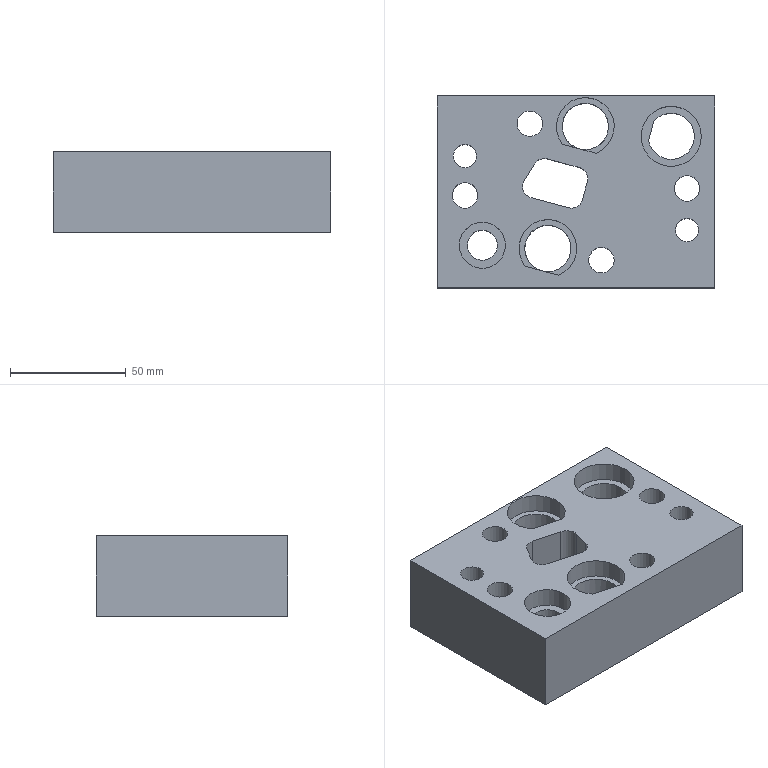Part | NX | features solid 2 | 1 solid | 47 faces | box 120 x 83 x 35 mm | volume 264601 mm3 | cylinder 24 | plane 23 | commonest cylinder face diameters 10 x6 11 x6 17 x4 20 x4 25 x2 13 x1
STEP:
#1=CARTESIAN_POINT('',(1378.149,-92.424,78.));
#2=VERTEX_POINT('',#1);
#3=CARTESIAN_POINT('',(1363.66,-88.542,78.));
#4=VERTEX_POINT('',#3);
#5=CARTESIAN_POINT('',(2014.625,-262.968,78.));
#6=DIRECTION('',(0.9659,-0.2588,0.));
#7=VECTOR('',#6,1000.);
#8=LINE('',#5,#7);
#9=EDGE_CURVE('',#2,#4,#8,.F.);
#10=ORIENTED_EDGE('',*,*,#9,.T.);
#11=CARTESIAN_POINT('',(1373.493,-80.824,78.));
#12=DIRECTION('',(0.,0.,-1.));
#13=DIRECTION('',(-1.,0.,0.));
#14=AXIS2_PLACEMENT_3D('',#11,#12,#13);
#15=CIRCLE('',#14,12.5);
#16=EDGE_CURVE('',#2,#4,#15,.F.);
#17=ORIENTED_EDGE('',*,*,#16,.F.);
#18=EDGE_LOOP('',(#10,#17));
#19=FACE_BOUND('',#18,.T.);
#20=CARTESIAN_POINT('',(1445.653,-14.891,78.));
#21=VERTEX_POINT('',#20);
#22=CARTESIAN_POINT('',(1325.653,-14.891,78.));
#23=VERTEX_POINT('',#22);
#24=CARTESIAN_POINT('',(1387.005,-14.891,78.));
#25=DIRECTION('',(1.,0.,0.));
#26=VECTOR('',#25,1000.);
#27=LINE('',#24,#26);
#28=EDGE_CURVE('',#21,#23,#27,.F.);
#29=ORIENTED_EDGE('',*,*,#28,.T.);
#30=CARTESIAN_POINT('',(1325.653,-97.891,78.));
#31=VERTEX_POINT('',#30);
#32=CARTESIAN_POINT('',(1325.653,-54.457,78.));
#33=DIRECTION('',(0.,1.,0.));
#34=VECTOR('',#33,1000.);
#35=LINE('',#32,#34);
#36=EDGE_CURVE('',#23,#31,#35,.F.);
#37=ORIENTED_EDGE('',*,*,#36,.T.);
#38=CARTESIAN_POINT('',(1445.653,-97.891,78.));
#39=VERTEX_POINT('',#38);
#40=CARTESIAN_POINT('',(1387.005,-97.891,78.));
#41=DIRECTION('',(-1.,0.,0.));
#42=VECTOR('',#41,1000.);
#43=LINE('',#40,#42);
#44=EDGE_CURVE('',#31,#39,#43,.F.);
#45=ORIENTED_EDGE('',*,*,#44,.T.);
#46=CARTESIAN_POINT('',(1445.653,-54.457,78.));
#47=DIRECTION('',(0.,-1.,0.));
#48=VECTOR('',#47,1000.);
#49=LINE('',#46,#48);
#50=EDGE_CURVE('',#39,#21,#49,.F.);
#51=ORIENTED_EDGE('',*,*,#50,.T.);
#52=EDGE_LOOP('',(#29,#37,#45,#51));
#53=FACE_BOUND('',#52,.T.);
#54=CARTESIAN_POINT('',(1439.153,-54.891,78.));
#55=VERTEX_POINT('',#54);
#56=CARTESIAN_POINT('',(1433.653,-54.891,78.));
#57=DIRECTION('',(0.,0.,-1.));
#58=DIRECTION('',(1.,0.,0.));
#59=AXIS2_PLACEMENT_3D('',#56,#57,#58);
#60=CIRCLE('',#59,5.5);
#61=EDGE_CURVE('',#55,#55,#60,.T.);
#62=ORIENTED_EDGE('',*,*,#61,.T.);
#63=EDGE_LOOP('',(#62));
#64=FACE_BOUND('',#63,.T.);
#65=CARTESIAN_POINT('',(1428.653,-72.891,78.));
#66=VERTEX_POINT('',#65);
#67=CARTESIAN_POINT('',(1433.653,-72.891,78.));
#68=DIRECTION('',(0.,0.,-1.));
#69=DIRECTION('',(-1.,0.,0.));
#70=AXIS2_PLACEMENT_3D('',#67,#68,#69);
#71=CIRCLE('',#70,5.);
#72=EDGE_CURVE('',#66,#66,#71,.T.);
#73=ORIENTED_EDGE('',*,*,#72,.T.);
#74=EDGE_LOOP('',(#73));
#75=FACE_BOUND('',#74,.T.);
#76=CARTESIAN_POINT('',(1413.856,-32.353,78.));
#77=VERTEX_POINT('',#76);
#78=CARTESIAN_POINT('',(1426.856,-32.353,78.));
#79=DIRECTION('',(0.,0.,-1.));
#80=DIRECTION('',(-1.,0.,0.));
#81=AXIS2_PLACEMENT_3D('',#78,#79,#80);
#82=CIRCLE('',#81,13.);
#83=EDGE_CURVE('',#77,#77,#82,.F.);
#84=ORIENTED_EDGE('',*,*,#83,.F.);
#85=EDGE_LOOP('',(#84));
#86=FACE_BOUND('',#85,.T.);
#87=CARTESIAN_POINT('',(1332.653,-40.891,78.));
#88=VERTEX_POINT('',#87);
#89=CARTESIAN_POINT('',(1337.653,-40.891,78.));
#90=DIRECTION('',(0.,0.,-1.));
#91=DIRECTION('',(-1.,0.,0.));
#92=AXIS2_PLACEMENT_3D('',#89,#90,#91);
#93=CIRCLE('',#92,5.);
#94=EDGE_CURVE('',#88,#88,#93,.T.);
#95=ORIENTED_EDGE('',*,*,#94,.T.);
#96=EDGE_LOOP('',(#95));
#97=FACE_BOUND('',#96,.T.);
#98=CARTESIAN_POINT('',(1402.153,-85.891,78.));
#99=VERTEX_POINT('',#98);
#100=CARTESIAN_POINT('',(1396.653,-85.891,78.));
#101=DIRECTION('',(0.,0.,-1.));
#102=DIRECTION('',(1.,0.,0.));
#103=AXIS2_PLACEMENT_3D('',#100,#101,#102);
#104=CIRCLE('',#103,5.5);
#105=EDGE_CURVE('',#99,#99,#104,.T.);
#106=ORIENTED_EDGE('',*,*,#105,.T.);
#107=EDGE_LOOP('',(#106));
#108=FACE_BOUND('',#107,.T.);
#109=CARTESIAN_POINT('',(1343.153,-57.891,78.));
#110=VERTEX_POINT('',#109);
#111=CARTESIAN_POINT('',(1337.653,-57.891,78.));
#112=DIRECTION('',(0.,0.,-1.));
#113=DIRECTION('',(1.,0.,0.));
#114=AXIS2_PLACEMENT_3D('',#111,#112,#113);
#115=CIRCLE('',#114,5.5);
#116=EDGE_CURVE('',#110,#110,#115,.T.);
#117=ORIENTED_EDGE('',*,*,#116,.T.);
#118=EDGE_LOOP('',(#117));
#119=FACE_BOUND('',#118,.T.);
#120=CARTESIAN_POINT('',(1371.153,-26.891,78.));
#121=VERTEX_POINT('',#120);
#122=CARTESIAN_POINT('',(1365.653,-26.891,78.));
#123=DIRECTION('',(0.,0.,-1.));
#124=DIRECTION('',(1.,0.,0.));
#125=AXIS2_PLACEMENT_3D('',#122,#123,#124);
#126=CIRCLE('',#125,5.5);
#127=EDGE_CURVE('',#121,#121,#126,.T.);
#128=ORIENTED_EDGE('',*,*,#127,.T.);
#129=EDGE_LOOP('',(#128));
#130=FACE_BOUND('',#129,.T.);
#131=CARTESIAN_POINT('',(1366.205,-58.89,78.));
#132=VERTEX_POINT('',#131);
#133=CARTESIAN_POINT('',(1382.352,-63.217,78.));
#134=VERTEX_POINT('',#133);
#135=CARTESIAN_POINT('',(2024.14,-235.184,78.));
#136=DIRECTION('',(0.9659,-0.2588,0.));
#137=VECTOR('',#136,1000.);
#138=LINE('',#135,#137);
#139=EDGE_CURVE('',#132,#134,#138,.T.);
#140=ORIENTED_EDGE('',*,*,#139,.F.);
#141=CARTESIAN_POINT('',(1363.259,-51.411,78.));
#142=VERTEX_POINT('',#141);
#143=CARTESIAN_POINT('',(1367.499,-54.061,78.));
#144=DIRECTION('',(0.,0.,1.));
#145=DIRECTION('',(-1.,0.,0.));
#146=AXIS2_PLACEMENT_3D('',#143,#144,#145);
#147=CIRCLE('',#146,5.);
#148=EDGE_CURVE('',#142,#132,#147,.T.);
#149=ORIENTED_EDGE('',*,*,#148,.F.);
#150=CARTESIAN_POINT('',(1367.692,-44.317,78.));
#151=VERTEX_POINT('',#150);
#152=CARTESIAN_POINT('',(1589.644,310.881,78.));
#153=DIRECTION('',(-0.5299,-0.848,0.));
#154=VECTOR('',#153,1000.);
#155=LINE('',#152,#154);
#156=EDGE_CURVE('',#151,#142,#155,.T.);
#157=ORIENTED_EDGE('',*,*,#156,.F.);
#158=CARTESIAN_POINT('',(1373.226,-42.137,78.));
#159=VERTEX_POINT('',#158);
#160=CARTESIAN_POINT('',(1371.932,-46.966,78.));
#161=DIRECTION('',(0.,0.,1.));
#162=DIRECTION('',(-1.,0.,0.));
#163=AXIS2_PLACEMENT_3D('',#160,#161,#162);
#164=CIRCLE('',#163,5.);
#165=EDGE_CURVE('',#159,#151,#164,.T.);
#166=ORIENTED_EDGE('',*,*,#165,.F.);
#167=CARTESIAN_POINT('',(1387.01,-45.83,78.));
#168=VERTEX_POINT('',#167);
#169=CARTESIAN_POINT('',(2028.799,-217.797,78.));
#170=DIRECTION('',(-0.9659,0.2588,0.));
#171=VECTOR('',#170,1000.);
#172=LINE('',#169,#171);
#173=EDGE_CURVE('',#168,#159,#172,.T.);
#174=ORIENTED_EDGE('',*,*,#173,.F.);
#175=CARTESIAN_POINT('',(1390.546,-51.954,78.));
#176=VERTEX_POINT('',#175);
#177=CARTESIAN_POINT('',(1385.716,-50.66,78.));
#178=DIRECTION('',(0.,0.,1.));
#179=DIRECTION('',(-1.,0.,0.));
#180=AXIS2_PLACEMENT_3D('',#177,#178,#179);
#181=CIRCLE('',#180,5.);
#182=EDGE_CURVE('',#176,#168,#181,.T.);
#183=ORIENTED_EDGE('',*,*,#182,.F.);
#184=CARTESIAN_POINT('',(1388.475,-59.681,78.));
#185=VERTEX_POINT('',#184);
#186=CARTESIAN_POINT('',(1450.198,170.673,78.));
#187=DIRECTION('',(0.2588,0.9659,0.));
#188=VECTOR('',#187,1000.);
#189=LINE('',#186,#188);
#190=EDGE_CURVE('',#185,#176,#189,.T.);
#191=ORIENTED_EDGE('',*,*,#190,.F.);
#192=CARTESIAN_POINT('',(1383.646,-58.387,78.));
#193=DIRECTION('',(0.,0.,1.));
#194=DIRECTION('',(-1.,0.,0.));
#195=AXIS2_PLACEMENT_3D('',#192,#193,#194);
#196=CIRCLE('',#195,5.);
#197=EDGE_CURVE('',#134,#185,#196,.T.);
#198=ORIENTED_EDGE('',*,*,#197,.F.);
#199=EDGE_LOOP('',(#140,#149,#157,#166,#174,#183,#191,#198));
#200=FACE_BOUND('',#199,.T.);
#201=CARTESIAN_POINT('',(1335.153,-79.442,78.));
#202=VERTEX_POINT('',#201);
#203=CARTESIAN_POINT('',(1345.153,-79.442,78.));
#204=DIRECTION('',(0.,0.,-1.));
#205=DIRECTION('',(-1.,0.,0.));
#206=AXIS2_PLACEMENT_3D('',#203,#204,#205);
#207=CIRCLE('',#206,10.);
#208=EDGE_CURVE('',#202,#202,#207,.F.);
#209=ORIENTED_EDGE('',*,*,#208,.F.);
#210=EDGE_LOOP('',(#209));
#211=FACE_BOUND('',#210,.T.);
#212=CARTESIAN_POINT('',(1394.35,-39.69,78.));
#213=VERTEX_POINT('',#212);
#214=CARTESIAN_POINT('',(1379.861,-35.807,78.));
#215=VERTEX_POINT('',#214);
#216=CARTESIAN_POINT('',(2030.826,-210.233,78.));
#217=DIRECTION('',(0.9659,-0.2588,0.));
#218=VECTOR('',#217,1000.);
#219=LINE('',#216,#218);
#220=EDGE_CURVE('',#213,#215,#219,.F.);
#221=ORIENTED_EDGE('',*,*,#220,.T.);
#222=CARTESIAN_POINT('',(1389.693,-28.089,78.));
#223=DIRECTION('',(0.,0.,-1.));
#224=DIRECTION('',(-1.,0.,0.));
#225=AXIS2_PLACEMENT_3D('',#222,#223,#224);
#226=CIRCLE('',#225,12.5);
#227=EDGE_CURVE('',#213,#215,#226,.F.);
#228=ORIENTED_EDGE('',*,*,#227,.F.);
#229=EDGE_LOOP('',(#221,#228));
#230=FACE_BOUND('',#229,.T.);
#231=CARTESIAN_POINT('',(2186.158,-0.000000688,78.));
#232=DIRECTION('',(0.,0.,-1.));
#233=DIRECTION('',(1.,0.,0.));
#234=AXIS2_PLACEMENT_3D('',#231,#232,#233);
#235=PLANE('',#234);
#236=ADVANCED_FACE('',(#19,#53,#64,#75,#86,#97,#108,#119,#130,#200,#211,#230),#235,.F.);
#237=CARTESIAN_POINT('',(1438.653,-72.891,53.));
#238=VERTEX_POINT('',#237);
#239=CARTESIAN_POINT('',(1433.653,-72.891,53.));
#240=DIRECTION('',(0.,0.,1.));
#241=DIRECTION('',(1.,0.,0.));
#242=AXIS2_PLACEMENT_3D('',#239,#240,#241);
#243=CIRCLE('',#242,5.);
#244=EDGE_CURVE('',#238,#238,#243,.T.);
#245=ORIENTED_EDGE('',*,*,#244,.T.);
#246=EDGE_LOOP('',(#245));
#247=FACE_BOUND('',#246,.T.);
#248=CARTESIAN_POINT('',(1439.153,-72.891,53.));
#249=VERTEX_POINT('',#248);
#250=CARTESIAN_POINT('',(1433.653,-72.891,53.));
#251=DIRECTION('',(0.,0.,-1.));
#252=DIRECTION('',(1.,0.,0.));
#253=AXIS2_PLACEMENT_3D('',#250,#251,#252);
#254=CIRCLE('',#253,5.5);
#255=EDGE_CURVE('',#249,#249,#254,.F.);
#256=ORIENTED_EDGE('',*,*,#255,.F.);
#257=EDGE_LOOP('',(#256));
#258=FACE_BOUND('',#257,.T.);
#259=CARTESIAN_POINT('',(1433.886,-74.397,53.));
#260=DIRECTION('',(0.,0.,1.));
#261=DIRECTION('',(1.,0.,0.));
#262=AXIS2_PLACEMENT_3D('',#259,#260,#261);
#263=PLANE('',#262);
#264=ADVANCED_FACE('',(#247,#258),#263,.F.);
#265=CARTESIAN_POINT('',(1439.153,-54.891,55.));
#266=VERTEX_POINT('',#265);
#267=CARTESIAN_POINT('',(1433.653,-54.891,55.));
#268=DIRECTION('',(0.,0.,-1.));
#269=DIRECTION('',(1.,0.,0.));
#270=AXIS2_PLACEMENT_3D('',#267,#268,#269);
#271=CIRCLE('',#270,5.5);
#272=EDGE_CURVE('',#266,#266,#271,.F.);
#273=ORIENTED_EDGE('',*,*,#272,.T.);
#274=EDGE_LOOP('',(#273));
#275=FACE_BOUND('',#274,.T.);
#276=CARTESIAN_POINT('',(1442.153,-54.891,55.));
#277=VERTEX_POINT('',#276);
#278=CARTESIAN_POINT('',(1433.653,-54.891,55.));
#279=DIRECTION('',(0.,0.,-1.));
#280=DIRECTION('',(1.,0.,0.));
#281=AXIS2_PLACEMENT_3D('',#278,#279,#280);
#282=CIRCLE('',#281,8.5);
#283=EDGE_CURVE('',#277,#277,#282,.F.);
#284=ORIENTED_EDGE('',*,*,#283,.F.);
#285=EDGE_LOOP('',(#284));
#286=FACE_BOUND('',#285,.T.);
#287=CARTESIAN_POINT('',(1431.945,-52.104,55.));
#288=DIRECTION('',(0.,0.,1.));
#289=DIRECTION('',(1.,0.,0.));
#290=AXIS2_PLACEMENT_3D('',#287,#288,#289);
#291=PLANE('',#290);
#292=ADVANCED_FACE('',(#275,#286),#291,.F.);
#293=ORIENTED_EDGE('',*,*,#72,.F.);
#294=EDGE_LOOP('',(#293));
#295=FACE_BOUND('',#294,.T.);
#296=ORIENTED_EDGE('',*,*,#244,.F.);
#297=EDGE_LOOP('',(#296));
#298=FACE_BOUND('',#297,.T.);
#299=CARTESIAN_POINT('',(1433.653,-72.891,78.));
#300=DIRECTION('',(0.,0.,1.));
#301=DIRECTION('',(1.,0.,0.));
#302=AXIS2_PLACEMENT_3D('',#299,#300,#301);
#303=CYLINDRICAL_SURFACE('',#302,5.);
#304=ADVANCED_FACE('',(#295,#298),#303,.F.);
#305=ORIENTED_EDGE('',*,*,#61,.F.);
#306=EDGE_LOOP('',(#305));
#307=FACE_BOUND('',#306,.T.);
#308=ORIENTED_EDGE('',*,*,#272,.F.);
#309=EDGE_LOOP('',(#308));
#310=FACE_BOUND('',#309,.T.);
#311=CARTESIAN_POINT('',(1433.653,-54.891,78.));
#312=DIRECTION('',(0.,0.,1.));
#313=DIRECTION('',(1.,0.,0.));
#314=AXIS2_PLACEMENT_3D('',#311,#312,#313);
#315=CYLINDRICAL_SURFACE('',#314,5.5);
#316=ADVANCED_FACE('',(#307,#310),#315,.F.);
#317=CARTESIAN_POINT('',(1445.653,-14.891,43.));
#318=VERTEX_POINT('',#317);
#319=CARTESIAN_POINT('',(1445.653,-97.891,43.));
#320=VERTEX_POINT('',#319);
#321=CARTESIAN_POINT('',(1445.653,-54.457,43.));
#322=DIRECTION('',(0.,-1.,0.));
#323=VECTOR('',#322,1000.);
#324=LINE('',#321,#323);
#325=EDGE_CURVE('',#318,#320,#324,.T.);
#326=ORIENTED_EDGE('',*,*,#325,.F.);
#327=CARTESIAN_POINT('',(1445.653,-14.891,60.));
#328=DIRECTION('',(0.,0.,1.));
#329=VECTOR('',#328,1000.);
#330=LINE('',#327,#329);
#331=EDGE_CURVE('',#318,#21,#330,.T.);
#332=ORIENTED_EDGE('',*,*,#331,.T.);
#333=ORIENTED_EDGE('',*,*,#50,.F.);
#334=CARTESIAN_POINT('',(1445.653,-97.891,60.));
#335=DIRECTION('',(0.,0.,1.));
#336=VECTOR('',#335,1000.);
#337=LINE('',#334,#336);
#338=EDGE_CURVE('',#320,#39,#337,.T.);
#339=ORIENTED_EDGE('',*,*,#338,.F.);
#340=EDGE_LOOP('',(#326,#332,#333,#339));
#341=FACE_BOUND('',#340,.T.);
#342=CARTESIAN_POINT('',(1445.653,-54.457,60.));
#343=DIRECTION('',(1.,0.,0.));
#344=DIRECTION('',(0.,0.,-1.));
#345=AXIS2_PLACEMENT_3D('',#342,#343,#344);
#346=PLANE('',#345);
#347=ADVANCED_FACE('',(#341),#346,.T.);
#348=ORIENTED_EDGE('',*,*,#255,.T.);
#349=EDGE_LOOP('',(#348));
#350=FACE_BOUND('',#349,.T.);
#351=CARTESIAN_POINT('',(1439.153,-72.891,43.));
#352=VERTEX_POINT('',#351);
#353=CARTESIAN_POINT('',(1433.653,-72.891,43.));
#354=DIRECTION('',(0.,0.,-1.));
#355=DIRECTION('',(1.,0.,0.));
#356=AXIS2_PLACEMENT_3D('',#353,#354,#355);
#357=CIRCLE('',#356,5.5);
#358=EDGE_CURVE('',#352,#352,#357,.T.);
#359=ORIENTED_EDGE('',*,*,#358,.T.);
#360=EDGE_LOOP('',(#359));
#361=FACE_BOUND('',#360,.T.);
#362=CARTESIAN_POINT('',(1433.653,-72.891,43.));
#363=DIRECTION('',(0.,0.,1.));
#364=DIRECTION('',(1.,0.,0.));
#365=AXIS2_PLACEMENT_3D('',#362,#363,#364);
#366=CYLINDRICAL_SURFACE('',#365,5.5);
#367=ADVANCED_FACE('',(#350,#361),#366,.F.);
#368=ORIENTED_EDGE('',*,*,#283,.T.);
#369=EDGE_LOOP('',(#368));
#370=FACE_BOUND('',#369,.T.);
#371=CARTESIAN_POINT('',(1442.153,-54.891,43.));
#372=VERTEX_POINT('',#371);
#373=CARTESIAN_POINT('',(1433.653,-54.891,43.));
#374=DIRECTION('',(0.,0.,-1.));
#375=DIRECTION('',(1.,0.,0.));
#376=AXIS2_PLACEMENT_3D('',#373,#374,#375);
#377=CIRCLE('',#376,8.5);
#378=EDGE_CURVE('',#372,#372,#377,.T.);
#379=ORIENTED_EDGE('',*,*,#378,.T.);
#380=EDGE_LOOP('',(#379));
#381=FACE_BOUND('',#380,.T.);
#382=CARTESIAN_POINT('',(1433.653,-54.891,43.));
#383=DIRECTION('',(0.,0.,1.));
#384=DIRECTION('',(1.,0.,0.));
#385=AXIS2_PLACEMENT_3D('',#382,#383,#384);
#386=CYLINDRICAL_SURFACE('',#385,8.5);
#387=ADVANCED_FACE('',(#370,#381),#386,.F.);
#388=CARTESIAN_POINT('',(1413.856,-32.353,69.8));
#389=VERTEX_POINT('',#388);
#390=CARTESIAN_POINT('',(1426.856,-32.353,69.8));
#391=DIRECTION('',(0.,0.,-1.));
#392=DIRECTION('',(-1.,0.,0.));
#393=AXIS2_PLACEMENT_3D('',#390,#391,#392);
#394=CIRCLE('',#393,13.);
#395=EDGE_CURVE('',#389,#389,#394,.T.);
#396=ORIENTED_EDGE('',*,*,#395,.F.);
#397=EDGE_LOOP('',(#396));
#398=FACE_BOUND('',#397,.T.);
#399=CARTESIAN_POINT('',(1417.035,-34.234,69.8));
#400=VERTEX_POINT('',#399);
#401=CARTESIAN_POINT('',(1419.291,-25.813,69.8));
#402=VERTEX_POINT('',#401);
#403=CARTESIAN_POINT('',(1426.856,-32.353,69.8));
#404=DIRECTION('',(0.,0.,1.));
#405=DIRECTION('',(-1.,0.,0.));
#406=AXIS2_PLACEMENT_3D('',#403,#404,#405);
#407=CIRCLE('',#406,10.);
#408=EDGE_CURVE('',#400,#402,#407,.T.);
#409=ORIENTED_EDGE('',*,*,#408,.F.);
#410=CARTESIAN_POINT('',(1470.483,165.237,69.8));
#411=DIRECTION('',(0.2588,0.9659,0.));
#412=VECTOR('',#411,1000.);
#413=LINE('',#410,#412);
#414=EDGE_CURVE('',#402,#400,#413,.F.);
#415=ORIENTED_EDGE('',*,*,#414,.F.);
#416=EDGE_LOOP('',(#409,#415));
#417=FACE_BOUND('',#416,.T.);
#418=CARTESIAN_POINT('',(2087.158,-0.000000688,69.8));
#419=DIRECTION('',(0.,0.,-1.));
#420=DIRECTION('',(1.,0.,0.));
#421=AXIS2_PLACEMENT_3D('',#418,#419,#420);
#422=PLANE('',#421);
#423=ADVANCED_FACE('',(#398,#417),#422,.F.);
#424=ORIENTED_EDGE('',*,*,#395,.T.);
#425=EDGE_LOOP('',(#424));
#426=FACE_BOUND('',#425,.T.);
#427=ORIENTED_EDGE('',*,*,#83,.T.);
#428=EDGE_LOOP('',(#427));
#429=FACE_BOUND('',#428,.T.);
#430=CARTESIAN_POINT('',(1426.856,-32.353,78.));
#431=DIRECTION('',(0.,0.,-1.));
#432=DIRECTION('',(-1.,0.,0.));
#433=AXIS2_PLACEMENT_3D('',#430,#431,#432);
#434=CYLINDRICAL_SURFACE('',#433,13.);
#435=ADVANCED_FACE('',(#426,#429),#434,.F.);
#436=CARTESIAN_POINT('',(1417.035,-34.234,43.));
#437=VERTEX_POINT('',#436);
#438=CARTESIAN_POINT('',(1417.035,-34.234,-21.4));
#439=DIRECTION('',(0.,0.,1.));
#440=VECTOR('',#439,1000.);
#441=LINE('',#438,#440);
#442=EDGE_CURVE('',#400,#437,#441,.F.);
#443=ORIENTED_EDGE('',*,*,#442,.F.);
#444=ORIENTED_EDGE('',*,*,#408,.T.);
#445=CARTESIAN_POINT('',(1419.291,-25.813,43.));
#446=VERTEX_POINT('',#445);
#447=CARTESIAN_POINT('',(1419.291,-25.813,-21.4));
#448=DIRECTION('',(0.,0.,1.));
#449=VECTOR('',#448,1000.);
#450=LINE('',#447,#449);
#451=EDGE_CURVE('',#446,#402,#450,.T.);
#452=ORIENTED_EDGE('',*,*,#451,.F.);
#453=CARTESIAN_POINT('',(1426.856,-32.353,43.));
#454=DIRECTION('',(0.,0.,1.));
#455=DIRECTION('',(-1.,0.,0.));
#456=AXIS2_PLACEMENT_3D('',#453,#454,#455);
#457=CIRCLE('',#456,10.);
#458=EDGE_CURVE('',#437,#446,#457,.T.);
#459=ORIENTED_EDGE('',*,*,#458,.F.);
#460=EDGE_LOOP('',(#443,#444,#452,#459));
#461=FACE_BOUND('',#460,.T.);
#462=CARTESIAN_POINT('',(1426.856,-32.353,-21.4));
#463=DIRECTION('',(0.,0.,1.));
#464=DIRECTION('',(1.,0.,0.));
#465=AXIS2_PLACEMENT_3D('',#462,#463,#464);
#466=CYLINDRICAL_SURFACE('',#465,10.);
#467=ADVANCED_FACE('',(#461),#466,.F.);
#468=CARTESIAN_POINT('',(1405.153,-85.891,43.));
#469=VERTEX_POINT('',#468);
#470=CARTESIAN_POINT('',(1396.653,-85.891,43.));
#471=DIRECTION('',(0.,0.,-1.));
#472=DIRECTION('',(1.,0.,0.));
#473=AXIS2_PLACEMENT_3D('',#470,#471,#472);
#474=CIRCLE('',#473,8.5);
#475=EDGE_CURVE('',#469,#469,#474,.T.);
#476=ORIENTED_EDGE('',*,*,#475,.T.);
#477=EDGE_LOOP('',(#476));
#478=FACE_BOUND('',#477,.T.);
#479=CARTESIAN_POINT('',(1405.153,-85.891,55.));
#480=VERTEX_POINT('',#479);
#481=CARTESIAN_POINT('',(1396.653,-85.891,55.));
#482=DIRECTION('',(0.,0.,-1.));
#483=DIRECTION('',(1.,0.,0.));
#484=AXIS2_PLACEMENT_3D('',#481,#482,#483);
#485=CIRCLE('',#484,8.5);
#486=EDGE_CURVE('',#480,#480,#485,.F.);
#487=ORIENTED_EDGE('',*,*,#486,.T.);
#488=EDGE_LOOP('',(#487));
#489=FACE_BOUND('',#488,.T.);
#490=CARTESIAN_POINT('',(1396.653,-85.891,43.));
#491=DIRECTION('',(0.,0.,1.));
#492=DIRECTION('',(1.,0.,0.));
#493=AXIS2_PLACEMENT_3D('',#490,#491,#492);
#494=CYLINDRICAL_SURFACE('',#493,8.5);
#495=ADVANCED_FACE('',(#478,#489),#494,.F.);
#496=ORIENTED_EDGE('',*,*,#486,.F.);
#497=EDGE_LOOP('',(#496));
#498=FACE_BOUND('',#497,.T.);
#499=CARTESIAN_POINT('',(1402.153,-85.891,55.));
#500=VERTEX_POINT('',#499);
#501=CARTESIAN_POINT('',(1396.653,-85.891,55.));
#502=DIRECTION('',(0.,0.,-1.));
#503=DIRECTION('',(1.,0.,0.));
#504=AXIS2_PLACEMENT_3D('',#501,#502,#503);
#505=CIRCLE('',#504,5.5);
#506=EDGE_CURVE('',#500,#500,#505,.F.);
#507=ORIENTED_EDGE('',*,*,#506,.T.);
#508=EDGE_LOOP('',(#507));
#509=FACE_BOUND('',#508,.T.);
#510=CARTESIAN_POINT('',(1397.063,-88.666,55.));
#511=DIRECTION('',(0.,0.,1.));
#512=DIRECTION('',(1.,0.,0.));
#513=AXIS2_PLACEMENT_3D('',#510,#511,#512);
#514=PLANE('',#513);
#515=ADVANCED_FACE('',(#498,#509),#514,.F.);
#516=CARTESIAN_POINT('',(1379.693,-28.089,43.));
#517=VERTEX_POINT('',#516);
#518=CARTESIAN_POINT('',(1389.693,-28.089,43.));
#519=DIRECTION('',(0.,0.,-1.));
#520=DIRECTION('',(-1.,0.,0.));
#521=AXIS2_PLACEMENT_3D('',#518,#519,#520);
#522=CIRCLE('',#521,10.);
#523=EDGE_CURVE('',#517,#517,#522,.T.);
#524=ORIENTED_EDGE('',*,*,#523,.F.);
#525=EDGE_LOOP('',(#524));
#526=FACE_BOUND('',#525,.T.);
#527=CARTESIAN_POINT('',(1363.493,-80.824,43.));
#528=VERTEX_POINT('',#527);
#529=CARTESIAN_POINT('',(1373.493,-80.824,43.));
#530=DIRECTION('',(0.,0.,-1.));
#531=DIRECTION('',(-1.,0.,0.));
#532=AXIS2_PLACEMENT_3D('',#529,#530,#531);
#533=CIRCLE('',#532,10.);
#534=EDGE_CURVE('',#528,#528,#533,.T.);
#535=ORIENTED_EDGE('',*,*,#534,.F.);
#536=EDGE_LOOP('',(#535));
#537=FACE_BOUND('',#536,.T.);
#538=CARTESIAN_POINT('',(1325.653,-97.891,43.));
#539=VERTEX_POINT('',#538);
#540=CARTESIAN_POINT('',(1325.653,-14.891,43.));
#541=VERTEX_POINT('',#540);
#542=CARTESIAN_POINT('',(1325.653,-54.457,43.));
#543=DIRECTION('',(0.,1.,0.));
#544=VECTOR('',#543,1000.);
#545=LINE('',#542,#544);
#546=EDGE_CURVE('',#539,#541,#545,.T.);
#547=ORIENTED_EDGE('',*,*,#546,.T.);
#548=CARTESIAN_POINT('',(1387.005,-14.891,43.));
#549=DIRECTION('',(1.,0.,0.));
#550=VECTOR('',#549,1000.);
#551=LINE('',#548,#550);
#552=EDGE_CURVE('',#541,#318,#551,.T.);
#553=ORIENTED_EDGE('',*,*,#552,.T.);
#554=ORIENTED_EDGE('',*,*,#325,.T.);
#555=CARTESIAN_POINT('',(1387.005,-97.891,43.));
#556=DIRECTION('',(-1.,0.,0.));
#557=VECTOR('',#556,1000.);
#558=LINE('',#555,#557);
#559=EDGE_CURVE('',#320,#539,#558,.T.);
#560=ORIENTED_EDGE('',*,*,#559,.T.);
#561=EDGE_LOOP('',(#547,#553,#554,#560));
#562=FACE_BOUND('',#561,.T.);
#563=ORIENTED_EDGE('',*,*,#475,.F.);
#564=EDGE_LOOP('',(#563));
#565=FACE_BOUND('',#564,.T.);
#566=ORIENTED_EDGE('',*,*,#378,.F.);
#567=EDGE_LOOP('',(#566));
#568=FACE_BOUND('',#567,.T.);
#569=ORIENTED_EDGE('',*,*,#358,.F.);
#570=EDGE_LOOP('',(#569));
#571=FACE_BOUND('',#570,.T.);
#572=ORIENTED_EDGE('',*,*,#458,.T.);
#573=CARTESIAN_POINT('',(1387.977,-142.68,43.));
#574=DIRECTION('',(0.2588,0.9659,0.));
#575=VECTOR('',#574,1000.);
#576=LINE('',#573,#575);
#577=EDGE_CURVE('',#446,#437,#576,.F.);
#578=ORIENTED_EDGE('',*,*,#577,.T.);
#579=EDGE_LOOP('',(#572,#578));
#580=FACE_BOUND('',#579,.T.);
#581=CARTESIAN_POINT('',(1343.153,-40.891,43.));
#582=VERTEX_POINT('',#581);
#583=CARTESIAN_POINT('',(1337.653,-40.891,43.));
#584=DIRECTION('',(0.,0.,-1.));
#585=DIRECTION('',(1.,0.,0.));
#586=AXIS2_PLACEMENT_3D('',#583,#584,#585);
#587=CIRCLE('',#586,5.5);
#588=EDGE_CURVE('',#582,#582,#587,.T.);
#589=ORIENTED_EDGE('',*,*,#588,.F.);
#590=EDGE_LOOP('',(#589));
#591=FACE_BOUND('',#590,.T.);
#592=CARTESIAN_POINT('',(1346.153,-57.891,43.));
#593=VERTEX_POINT('',#592);
#594=CARTESIAN_POINT('',(1337.653,-57.891,43.));
#595=DIRECTION('',(0.,0.,-1.));
#596=DIRECTION('',(1.,0.,0.));
#597=AXIS2_PLACEMENT_3D('',#594,#595,#596);
#598=CIRCLE('',#597,8.5);
#599=EDGE_CURVE('',#593,#593,#598,.T.);
#600=ORIENTED_EDGE('',*,*,#599,.F.);
#601=EDGE_LOOP('',(#600));
#602=FACE_BOUND('',#601,.T.);
#603=CARTESIAN_POINT('',(1374.153,-26.891,43.));
#604=VERTEX_POINT('',#603);
#605=CARTESIAN_POINT('',(1365.653,-26.891,43.));
#606=DIRECTION('',(0.,0.,-1.));
#607=DIRECTION('',(1.,0.,0.));
#608=AXIS2_PLACEMENT_3D('',#605,#606,#607);
#609=CIRCLE('',#608,8.5);
#610=EDGE_CURVE('',#604,#604,#609,.T.);
#611=ORIENTED_EDGE('',*,*,#610,.F.);
#612=EDGE_LOOP('',(#611));
#613=FACE_BOUND('',#612,.T.);
#614=CARTESIAN_POINT('',(1366.205,-58.89,43.));
#615=VERTEX_POINT('',#614);
#616=CARTESIAN_POINT('',(1382.352,-63.217,43.));
#617=VERTEX_POINT('',#616);
#618=CARTESIAN_POINT('',(1404.568,-69.17,43.));
#619=DIRECTION('',(0.9659,-0.2588,0.));
#620=VECTOR('',#619,1000.);
#621=LINE('',#618,#620);
#622=EDGE_CURVE('',#615,#617,#621,.T.);
#623=ORIENTED_EDGE('',*,*,#622,.T.);
#624=CARTESIAN_POINT('',(1388.475,-59.681,43.));
#625=VERTEX_POINT('',#624);
#626=CARTESIAN_POINT('',(1383.646,-58.387,43.));
#627=DIRECTION('',(0.,0.,1.));
#628=DIRECTION('',(-1.,0.,0.));
#629=AXIS2_PLACEMENT_3D('',#626,#627,#628);
#630=CIRCLE('',#629,5.);
#631=EDGE_CURVE('',#617,#625,#630,.T.);
#632=ORIENTED_EDGE('',*,*,#631,.T.);
#633=CARTESIAN_POINT('',(1390.546,-51.954,43.));
#634=VERTEX_POINT('',#633);
#635=CARTESIAN_POINT('',(1367.692,-137.245,43.));
#636=DIRECTION('',(0.2588,0.9659,0.));
#637=VECTOR('',#636,1000.);
#638=LINE('',#635,#637);
#639=EDGE_CURVE('',#625,#634,#638,.T.);
#640=ORIENTED_EDGE('',*,*,#639,.T.);
#641=CARTESIAN_POINT('',(1387.01,-45.83,43.));
#642=VERTEX_POINT('',#641);
#643=CARTESIAN_POINT('',(1385.716,-50.66,43.));
#644=DIRECTION('',(0.,0.,1.));
#645=DIRECTION('',(-1.,0.,0.));
#646=AXIS2_PLACEMENT_3D('',#643,#644,#645);
#647=CIRCLE('',#646,5.);
#648=EDGE_CURVE('',#634,#642,#647,.T.);
#649=ORIENTED_EDGE('',*,*,#648,.T.);
#650=CARTESIAN_POINT('',(1373.226,-42.137,43.));
#651=VERTEX_POINT('',#650);
#652=CARTESIAN_POINT('',(1409.227,-51.783,43.));
#653=DIRECTION('',(-0.9659,0.2588,0.));
#654=VECTOR('',#653,1000.);
#655=LINE('',#652,#654);
#656=EDGE_CURVE('',#642,#651,#655,.T.);
#657=ORIENTED_EDGE('',*,*,#656,.T.);
#658=CARTESIAN_POINT('',(1367.692,-44.317,43.));
#659=VERTEX_POINT('',#658);
#660=CARTESIAN_POINT('',(1371.932,-46.966,43.));
#661=DIRECTION('',(0.,0.,1.));
#662=DIRECTION('',(-1.,0.,0.));
#663=AXIS2_PLACEMENT_3D('',#660,#661,#662);
#664=CIRCLE('',#663,5.);
#665=EDGE_CURVE('',#651,#659,#664,.T.);
#666=ORIENTED_EDGE('',*,*,#665,.T.);
#667=CARTESIAN_POINT('',(1363.259,-51.411,43.));
#668=VERTEX_POINT('',#667);
#669=CARTESIAN_POINT('',(1328.719,-106.686,43.));
#670=DIRECTION('',(-0.5299,-0.848,0.));
#671=VECTOR('',#670,1000.);
#672=LINE('',#669,#671);
#673=EDGE_CURVE('',#659,#668,#672,.T.);
#674=ORIENTED_EDGE('',*,*,#673,.T.);
#675=CARTESIAN_POINT('',(1367.499,-54.061,43.));
#676=DIRECTION('',(0.,0.,1.));
#677=DIRECTION('',(-1.,0.,0.));
#678=AXIS2_PLACEMENT_3D('',#675,#676,#677);
#679=CIRCLE('',#678,5.);
#680=EDGE_CURVE('',#668,#615,#679,.T.);
#681=ORIENTED_EDGE('',*,*,#680,.T.);
#682=EDGE_LOOP('',(#623,#632,#640,#649,#657,#666,#674,#681));
#683=FACE_BOUND('',#682,.T.);
#684=CARTESIAN_POINT('',(1338.653,-79.442,43.));
#685=VERTEX_POINT('',#684);
#686=CARTESIAN_POINT('',(1345.153,-79.442,43.));
#687=DIRECTION('',(0.,0.,-1.));
#688=DIRECTION('',(-1.,0.,0.));
#689=AXIS2_PLACEMENT_3D('',#686,#687,#688);
#690=CIRCLE('',#689,6.5);
#691=EDGE_CURVE('',#685,#685,#690,.F.);
#692=ORIENTED_EDGE('',*,*,#691,.T.);
#693=EDGE_LOOP('',(#692));
#694=FACE_BOUND('',#693,.T.);
#695=CARTESIAN_POINT('',(1385.079,-141.904,43.));
#696=DIRECTION('',(0.,0.,-1.));
#697=DIRECTION('',(1.,0.,0.));
#698=AXIS2_PLACEMENT_3D('',#695,#696,#697);
#699=PLANE('',#698);
#700=ADVANCED_FACE('',(#526,#537,#562,#565,#568,#571,#580,#591,#602,#613,#683,#694),#699,.T.);
#701=ORIENTED_EDGE('',*,*,#44,.F.);
#702=CARTESIAN_POINT('',(1325.653,-97.891,60.));
#703=DIRECTION('',(0.,0.,1.));
#704=VECTOR('',#703,1000.);
#705=LINE('',#702,#704);
#706=EDGE_CURVE('',#539,#31,#705,.T.);
#707=ORIENTED_EDGE('',*,*,#706,.F.);
#708=ORIENTED_EDGE('',*,*,#559,.F.);
#709=ORIENTED_EDGE('',*,*,#338,.T.);
#710=EDGE_LOOP('',(#701,#707,#708,#709));
#711=FACE_BOUND('',#710,.T.);
#712=CARTESIAN_POINT('',(1387.005,-97.891,60.));
#713=DIRECTION('',(0.,-1.,0.));
#714=DIRECTION('',(0.,0.,1.));
#715=AXIS2_PLACEMENT_3D('',#712,#713,#714);
#716=PLANE('',#715);
#717=ADVANCED_FACE('',(#711),#716,.T.);
#718=ORIENTED_EDGE('',*,*,#552,.F.);
#719=CARTESIAN_POINT('',(1325.653,-14.891,60.));
#720=DIRECTION('',(0.,0.,1.));
#721=VECTOR('',#720,1000.);
#722=LINE('',#719,#721);
#723=EDGE_CURVE('',#541,#23,#722,.T.);
#724=ORIENTED_EDGE('',*,*,#723,.T.);
#725=ORIENTED_EDGE('',*,*,#28,.F.);
#726=ORIENTED_EDGE('',*,*,#331,.F.);
#727=EDGE_LOOP('',(#718,#724,#725,#726));
#728=FACE_BOUND('',#727,.T.);
#729=CARTESIAN_POINT('',(1387.005,-14.891,60.));
#730=DIRECTION('',(0.,1.,0.));
#731=DIRECTION('',(0.,0.,-1.));
#732=AXIS2_PLACEMENT_3D('',#729,#730,#731);
#733=PLANE('',#732);
#734=ADVANCED_FACE('',(#728),#733,.T.);
#735=ORIENTED_EDGE('',*,*,#577,.F.);
#736=ORIENTED_EDGE('',*,*,#451,.T.);
#737=ORIENTED_EDGE('',*,*,#414,.T.);
#738=ORIENTED_EDGE('',*,*,#442,.T.);
#739=EDGE_LOOP('',(#735,#736,#737,#738));
#740=FACE_BOUND('',#739,.T.);
#741=CARTESIAN_POINT('',(1418.163,-30.024,44.472));
#742=DIRECTION('',(-0.9659,0.2588,0.));
#743=DIRECTION('',(-0.2588,-0.9659,0.));
#744=AXIS2_PLACEMENT_3D('',#741,#742,#743);
#745=PLANE('',#744);
#746=ADVANCED_FACE('',(#740),#745,.F.);
#747=ORIENTED_EDGE('',*,*,#723,.F.);
#748=ORIENTED_EDGE('',*,*,#546,.F.);
#749=ORIENTED_EDGE('',*,*,#706,.T.);
#750=ORIENTED_EDGE('',*,*,#36,.F.);
#751=EDGE_LOOP('',(#747,#748,#749,#750));
#752=FACE_BOUND('',#751,.T.);
#753=CARTESIAN_POINT('',(1325.653,-54.457,60.));
#754=DIRECTION('',(-1.,0.,0.));
#755=DIRECTION('',(0.,0.,1.));
#756=AXIS2_PLACEMENT_3D('',#753,#754,#755);
#757=PLANE('',#756);
#758=ADVANCED_FACE('',(#752),#757,.T.);
#759=ORIENTED_EDGE('',*,*,#691,.F.);
#760=EDGE_LOOP('',(#759));
#761=FACE_BOUND('',#760,.T.);
#762=CARTESIAN_POINT('',(1338.653,-79.442,69.8));
#763=VERTEX_POINT('',#762);
#764=CARTESIAN_POINT('',(1345.153,-79.442,69.8));
#765=DIRECTION('',(0.,0.,-1.));
#766=DIRECTION('',(-1.,0.,0.));
#767=AXIS2_PLACEMENT_3D('',#764,#765,#766);
#768=CIRCLE('',#767,6.5);
#769=EDGE_CURVE('',#763,#763,#768,.F.);
#770=ORIENTED_EDGE('',*,*,#769,.T.);
#771=EDGE_LOOP('',(#770));
#772=FACE_BOUND('',#771,.T.);
#773=CARTESIAN_POINT('',(1345.153,-79.442,80.982));
#774=DIRECTION('',(0.,0.,-1.));
#775=DIRECTION('',(-1.,0.,0.));
#776=AXIS2_PLACEMENT_3D('',#773,#774,#775);
#777=CYLINDRICAL_SURFACE('',#776,6.5);
#778=ADVANCED_FACE('',(#761,#772),#777,.F.);
#779=ORIENTED_EDGE('',*,*,#208,.T.);
#780=EDGE_LOOP('',(#779));
#781=FACE_BOUND('',#780,.T.);
#782=CARTESIAN_POINT('',(1335.153,-79.442,69.8));
#783=VERTEX_POINT('',#782);
#784=CARTESIAN_POINT('',(1345.153,-79.442,69.8));
#785=DIRECTION('',(0.,0.,-1.));
#786=DIRECTION('',(-1.,0.,0.));
#787=AXIS2_PLACEMENT_3D('',#784,#785,#786);
#788=CIRCLE('',#787,10.);
#789=EDGE_CURVE('',#783,#783,#788,.T.);
#790=ORIENTED_EDGE('',*,*,#789,.T.);
#791=EDGE_LOOP('',(#790));
#792=FACE_BOUND('',#791,.T.);
#793=CARTESIAN_POINT('',(1345.153,-79.442,78.));
#794=DIRECTION('',(0.,0.,-1.));
#795=DIRECTION('',(-1.,0.,0.));
#796=AXIS2_PLACEMENT_3D('',#793,#794,#795);
#797=CYLINDRICAL_SURFACE('',#796,10.);
#798=ADVANCED_FACE('',(#781,#792),#797,.F.);
#799=ORIENTED_EDGE('',*,*,#769,.F.);
#800=EDGE_LOOP('',(#799));
#801=FACE_BOUND('',#800,.T.);
#802=ORIENTED_EDGE('',*,*,#789,.F.);
#803=EDGE_LOOP('',(#802));
#804=FACE_BOUND('',#803,.T.);
#805=CARTESIAN_POINT('',(2087.158,-0.000000688,69.8));
#806=DIRECTION('',(0.,0.,-1.));
#807=DIRECTION('',(1.,0.,0.));
#808=AXIS2_PLACEMENT_3D('',#805,#806,#807);
#809=PLANE('',#808);
#810=ADVANCED_FACE('',(#801,#804),#809,.F.);
#811=ORIENTED_EDGE('',*,*,#680,.F.);
#812=CARTESIAN_POINT('',(1363.259,-51.411,82.));
#813=DIRECTION('',(0.,0.,-1.));
#814=VECTOR('',#813,1000.);
#815=LINE('',#812,#814);
#816=EDGE_CURVE('',#668,#142,#815,.F.);
#817=ORIENTED_EDGE('',*,*,#816,.T.);
#818=ORIENTED_EDGE('',*,*,#148,.T.);
#819=CARTESIAN_POINT('',(1366.205,-58.89,82.));
#820=DIRECTION('',(0.,0.,-1.));
#821=VECTOR('',#820,1000.);
#822=LINE('',#819,#821);
#823=EDGE_CURVE('',#615,#132,#822,.F.);
#824=ORIENTED_EDGE('',*,*,#823,.F.);
#825=EDGE_LOOP('',(#811,#817,#818,#824));
#826=FACE_BOUND('',#825,.T.);
#827=CARTESIAN_POINT('',(1367.499,-54.061,82.));
#828=DIRECTION('',(0.,0.,-1.));
#829=DIRECTION('',(-1.,0.,0.));
#830=AXIS2_PLACEMENT_3D('',#827,#828,#829);
#831=CYLINDRICAL_SURFACE('',#830,5.);
#832=ADVANCED_FACE('',(#826),#831,.F.);
#833=ORIENTED_EDGE('',*,*,#673,.F.);
#834=CARTESIAN_POINT('',(1367.692,-44.317,82.));
#835=DIRECTION('',(0.,0.,-1.));
#836=VECTOR('',#835,1000.);
#837=LINE('',#834,#836);
#838=EDGE_CURVE('',#659,#151,#837,.F.);
#839=ORIENTED_EDGE('',*,*,#838,.T.);
#840=ORIENTED_EDGE('',*,*,#156,.T.);
#841=ORIENTED_EDGE('',*,*,#816,.F.);
#842=EDGE_LOOP('',(#833,#839,#840,#841));
#843=FACE_BOUND('',#842,.T.);
#844=CARTESIAN_POINT('',(1367.692,-44.317,82.));
#845=DIRECTION('',(-0.848,0.5299,0.));
#846=DIRECTION('',(0.5299,0.848,0.));
#847=AXIS2_PLACEMENT_3D('',#844,#845,#846);
#848=PLANE('',#847);
#849=ADVANCED_FACE('',(#843),#848,.F.);
#850=ORIENTED_EDGE('',*,*,#665,.F.);
#851=CARTESIAN_POINT('',(1373.226,-42.137,82.));
#852=DIRECTION('',(0.,0.,-1.));
#853=VECTOR('',#852,1000.);
#854=LINE('',#851,#853);
#855=EDGE_CURVE('',#651,#159,#854,.F.);
#856=ORIENTED_EDGE('',*,*,#855,.T.);
#857=ORIENTED_EDGE('',*,*,#165,.T.);
#858=ORIENTED_EDGE('',*,*,#838,.F.);
#859=EDGE_LOOP('',(#850,#856,#857,#858));
#860=FACE_BOUND('',#859,.T.);
#861=CARTESIAN_POINT('',(1371.932,-46.966,82.));
#862=DIRECTION('',(0.,0.,-1.));
#863=DIRECTION('',(-1.,0.,0.));
#864=AXIS2_PLACEMENT_3D('',#861,#862,#863);
#865=CYLINDRICAL_SURFACE('',#864,5.);
#866=ADVANCED_FACE('',(#860),#865,.F.);
#867=ORIENTED_EDGE('',*,*,#656,.F.);
#868=CARTESIAN_POINT('',(1387.01,-45.83,82.));
#869=DIRECTION('',(0.,0.,-1.));
#870=VECTOR('',#869,1000.);
#871=LINE('',#868,#870);
#872=EDGE_CURVE('',#642,#168,#871,.F.);
#873=ORIENTED_EDGE('',*,*,#872,.T.);
#874=ORIENTED_EDGE('',*,*,#173,.T.);
#875=ORIENTED_EDGE('',*,*,#855,.F.);
#876=EDGE_LOOP('',(#867,#873,#874,#875));
#877=FACE_BOUND('',#876,.T.);
#878=CARTESIAN_POINT('',(1387.01,-45.83,82.));
#879=DIRECTION('',(0.2588,0.9659,0.));
#880=DIRECTION('',(0.9659,-0.2588,0.));
#881=AXIS2_PLACEMENT_3D('',#878,#879,#880);
#882=PLANE('',#881);
#883=ADVANCED_FACE('',(#877),#882,.F.);
#884=ORIENTED_EDGE('',*,*,#648,.F.);
#885=CARTESIAN_POINT('',(1390.546,-51.954,82.));
#886=DIRECTION('',(0.,0.,-1.));
#887=VECTOR('',#886,1000.);
#888=LINE('',#885,#887);
#889=EDGE_CURVE('',#634,#176,#888,.F.);
#890=ORIENTED_EDGE('',*,*,#889,.T.);
#891=ORIENTED_EDGE('',*,*,#182,.T.);
#892=ORIENTED_EDGE('',*,*,#872,.F.);
#893=EDGE_LOOP('',(#884,#890,#891,#892));
#894=FACE_BOUND('',#893,.T.);
#895=CARTESIAN_POINT('',(1385.716,-50.66,82.));
#896=DIRECTION('',(0.,0.,-1.));
#897=DIRECTION('',(-1.,0.,0.));
#898=AXIS2_PLACEMENT_3D('',#895,#896,#897);
#899=CYLINDRICAL_SURFACE('',#898,5.);
#900=ADVANCED_FACE('',(#894),#899,.F.);
#901=ORIENTED_EDGE('',*,*,#639,.F.);
#902=CARTESIAN_POINT('',(1388.475,-59.681,82.));
#903=DIRECTION('',(0.,0.,-1.));
#904=VECTOR('',#903,1000.);
#905=LINE('',#902,#904);
#906=EDGE_CURVE('',#625,#185,#905,.F.);
#907=ORIENTED_EDGE('',*,*,#906,.T.);
#908=ORIENTED_EDGE('',*,*,#190,.T.);
#909=ORIENTED_EDGE('',*,*,#889,.F.);
#910=EDGE_LOOP('',(#901,#907,#908,#909));
#911=FACE_BOUND('',#910,.T.);
#912=CARTESIAN_POINT('',(1388.475,-59.681,82.));
#913=DIRECTION('',(0.9659,-0.2588,0.));
#914=DIRECTION('',(-0.2588,-0.9659,0.));
#915=AXIS2_PLACEMENT_3D('',#912,#913,#914);
#916=PLANE('',#915);
#917=ADVANCED_FACE('',(#911),#916,.F.);
#918=ORIENTED_EDGE('',*,*,#631,.F.);
#919=CARTESIAN_POINT('',(1382.352,-63.217,82.));
#920=DIRECTION('',(0.,0.,-1.));
#921=VECTOR('',#920,1000.);
#922=LINE('',#919,#921);
#923=EDGE_CURVE('',#617,#134,#922,.F.);
#924=ORIENTED_EDGE('',*,*,#923,.T.);
#925=ORIENTED_EDGE('',*,*,#197,.T.);
#926=ORIENTED_EDGE('',*,*,#906,.F.);
#927=EDGE_LOOP('',(#918,#924,#925,#926));
#928=FACE_BOUND('',#927,.T.);
#929=CARTESIAN_POINT('',(1383.646,-58.387,82.));
#930=DIRECTION('',(0.,0.,-1.));
#931=DIRECTION('',(-1.,0.,0.));
#932=AXIS2_PLACEMENT_3D('',#929,#930,#931);
#933=CYLINDRICAL_SURFACE('',#932,5.);
#934=ADVANCED_FACE('',(#928),#933,.F.);
#935=ORIENTED_EDGE('',*,*,#622,.F.);
#936=ORIENTED_EDGE('',*,*,#823,.T.);
#937=ORIENTED_EDGE('',*,*,#139,.T.);
#938=ORIENTED_EDGE('',*,*,#923,.F.);
#939=EDGE_LOOP('',(#935,#936,#937,#938));
#940=FACE_BOUND('',#939,.T.);
#941=CARTESIAN_POINT('',(1366.205,-58.89,82.));
#942=DIRECTION('',(-0.2588,-0.9659,0.));
#943=DIRECTION('',(-0.9659,0.2588,0.));
#944=AXIS2_PLACEMENT_3D('',#941,#942,#943);
#945=PLANE('',#944);
#946=ADVANCED_FACE('',(#940),#945,.F.);
#947=ORIENTED_EDGE('',*,*,#127,.F.);
#948=EDGE_LOOP('',(#947));
#949=FACE_BOUND('',#948,.T.);
#950=CARTESIAN_POINT('',(1371.153,-26.891,55.));
#951=VERTEX_POINT('',#950);
#952=CARTESIAN_POINT('',(1365.653,-26.891,55.));
#953=DIRECTION('',(0.,0.,-1.));
#954=DIRECTION('',(1.,0.,0.));
#955=AXIS2_PLACEMENT_3D('',#952,#953,#954);
#956=CIRCLE('',#955,5.5);
#957=EDGE_CURVE('',#951,#951,#956,.F.);
#958=ORIENTED_EDGE('',*,*,#957,.F.);
#959=EDGE_LOOP('',(#958));
#960=FACE_BOUND('',#959,.T.);
#961=CARTESIAN_POINT('',(1365.653,-26.891,78.));
#962=DIRECTION('',(0.,0.,1.));
#963=DIRECTION('',(1.,0.,0.));
#964=AXIS2_PLACEMENT_3D('',#961,#962,#963);
#965=CYLINDRICAL_SURFACE('',#964,5.5);
#966=ADVANCED_FACE('',(#949,#960),#965,.F.);
#967=ORIENTED_EDGE('',*,*,#957,.T.);
#968=EDGE_LOOP('',(#967));
#969=FACE_BOUND('',#968,.T.);
#970=CARTESIAN_POINT('',(1374.153,-26.891,55.));
#971=VERTEX_POINT('',#970);
#972=CARTESIAN_POINT('',(1365.653,-26.891,55.));
#973=DIRECTION('',(0.,0.,-1.));
#974=DIRECTION('',(1.,0.,0.));
#975=AXIS2_PLACEMENT_3D('',#972,#973,#974);
#976=CIRCLE('',#975,8.5);
#977=EDGE_CURVE('',#971,#971,#976,.F.);
#978=ORIENTED_EDGE('',*,*,#977,.F.);
#979=EDGE_LOOP('',(#978));
#980=FACE_BOUND('',#979,.T.);
#981=CARTESIAN_POINT('',(1367.2,-28.017,55.));
#982=DIRECTION('',(0.,0.,1.));
#983=DIRECTION('',(1.,0.,0.));
#984=AXIS2_PLACEMENT_3D('',#981,#982,#983);
#985=PLANE('',#984);
#986=ADVANCED_FACE('',(#969,#980),#985,.F.);
#987=ORIENTED_EDGE('',*,*,#977,.T.);
#988=EDGE_LOOP('',(#987));
#989=FACE_BOUND('',#988,.T.);
#990=ORIENTED_EDGE('',*,*,#610,.T.);
#991=EDGE_LOOP('',(#990));
#992=FACE_BOUND('',#991,.T.);
#993=CARTESIAN_POINT('',(1365.653,-26.891,43.));
#994=DIRECTION('',(0.,0.,1.));
#995=DIRECTION('',(1.,0.,0.));
#996=AXIS2_PLACEMENT_3D('',#993,#994,#995);
#997=CYLINDRICAL_SURFACE('',#996,8.5);
#998=ADVANCED_FACE('',(#989,#992),#997,.F.);
#999=ORIENTED_EDGE('',*,*,#116,.F.);
#1000=EDGE_LOOP('',(#999));
#1001=FACE_BOUND('',#1000,.T.);
#1002=CARTESIAN_POINT('',(1343.153,-57.891,55.));
#1003=VERTEX_POINT('',#1002);
#1004=CARTESIAN_POINT('',(1337.653,-57.891,55.));
#1005=DIRECTION('',(0.,0.,-1.));
#1006=DIRECTION('',(1.,0.,0.));
#1007=AXIS2_PLACEMENT_3D('',#1004,#1005,#1006);
#1008=CIRCLE('',#1007,5.5);
#1009=EDGE_CURVE('',#1003,#1003,#1008,.F.);
#1010=ORIENTED_EDGE('',*,*,#1009,.F.);
#1011=EDGE_LOOP('',(#1010));
#1012=FACE_BOUND('',#1011,.T.);
#1013=CARTESIAN_POINT('',(1337.653,-57.891,78.));
#1014=DIRECTION('',(0.,0.,1.));
#1015=DIRECTION('',(1.,0.,0.));
#1016=AXIS2_PLACEMENT_3D('',#1013,#1014,#1015);
#1017=CYLINDRICAL_SURFACE('',#1016,5.5);
#1018=ADVANCED_FACE('',(#1001,#1012),#1017,.F.);
#1019=ORIENTED_EDGE('',*,*,#1009,.T.);
#1020=EDGE_LOOP('',(#1019));
#1021=FACE_BOUND('',#1020,.T.);
#1022=CARTESIAN_POINT('',(1346.153,-57.891,55.));
#1023=VERTEX_POINT('',#1022);
#1024=CARTESIAN_POINT('',(1337.653,-57.891,55.));
#1025=DIRECTION('',(0.,0.,-1.));
#1026=DIRECTION('',(1.,0.,0.));
#1027=AXIS2_PLACEMENT_3D('',#1024,#1025,#1026);
#1028=CIRCLE('',#1027,8.5);
#1029=EDGE_CURVE('',#1023,#1023,#1028,.F.);
#1030=ORIENTED_EDGE('',*,*,#1029,.F.);
#1031=EDGE_LOOP('',(#1030));
#1032=FACE_BOUND('',#1031,.T.);
#1033=CARTESIAN_POINT('',(1336.284,-59.381,55.));
#1034=DIRECTION('',(0.,0.,1.));
#1035=DIRECTION('',(1.,0.,0.));
#1036=AXIS2_PLACEMENT_3D('',#1033,#1034,#1035);
#1037=PLANE('',#1036);
#1038=ADVANCED_FACE('',(#1021,#1032),#1037,.F.);
#1039=ORIENTED_EDGE('',*,*,#1029,.T.);
#1040=EDGE_LOOP('',(#1039));
#1041=FACE_BOUND('',#1040,.T.);
#1042=ORIENTED_EDGE('',*,*,#599,.T.);
#1043=EDGE_LOOP('',(#1042));
#1044=FACE_BOUND('',#1043,.T.);
#1045=CARTESIAN_POINT('',(1337.653,-57.891,43.));
#1046=DIRECTION('',(0.,0.,1.));
#1047=DIRECTION('',(1.,0.,0.));
#1048=AXIS2_PLACEMENT_3D('',#1045,#1046,#1047);
#1049=CYLINDRICAL_SURFACE('',#1048,8.5);
#1050=ADVANCED_FACE('',(#1041,#1044),#1049,.F.);
#1051=ORIENTED_EDGE('',*,*,#105,.F.);
#1052=EDGE_LOOP('',(#1051));
#1053=FACE_BOUND('',#1052,.T.);
#1054=ORIENTED_EDGE('',*,*,#506,.F.);
#1055=EDGE_LOOP('',(#1054));
#1056=FACE_BOUND('',#1055,.T.);
#1057=CARTESIAN_POINT('',(1396.653,-85.891,78.));
#1058=DIRECTION('',(0.,0.,1.));
#1059=DIRECTION('',(1.,0.,0.));
#1060=AXIS2_PLACEMENT_3D('',#1057,#1058,#1059);
#1061=CYLINDRICAL_SURFACE('',#1060,5.5);
#1062=ADVANCED_FACE('',(#1053,#1056),#1061,.F.);
#1063=ORIENTED_EDGE('',*,*,#94,.F.);
#1064=EDGE_LOOP('',(#1063));
#1065=FACE_BOUND('',#1064,.T.);
#1066=CARTESIAN_POINT('',(1342.653,-40.891,53.));
#1067=VERTEX_POINT('',#1066);
#1068=CARTESIAN_POINT('',(1337.653,-40.891,53.));
#1069=DIRECTION('',(0.,0.,1.));
#1070=DIRECTION('',(1.,0.,0.));
#1071=AXIS2_PLACEMENT_3D('',#1068,#1069,#1070);
#1072=CIRCLE('',#1071,5.);
#1073=EDGE_CURVE('',#1067,#1067,#1072,.T.);
#1074=ORIENTED_EDGE('',*,*,#1073,.F.);
#1075=EDGE_LOOP('',(#1074));
#1076=FACE_BOUND('',#1075,.T.);
#1077=CARTESIAN_POINT('',(1337.653,-40.891,78.));
#1078=DIRECTION('',(0.,0.,1.));
#1079=DIRECTION('',(1.,0.,0.));
#1080=AXIS2_PLACEMENT_3D('',#1077,#1078,#1079);
#1081=CYLINDRICAL_SURFACE('',#1080,5.);
#1082=ADVANCED_FACE('',(#1065,#1076),#1081,.F.);
#1083=ORIENTED_EDGE('',*,*,#1073,.T.);
#1084=EDGE_LOOP('',(#1083));
#1085=FACE_BOUND('',#1084,.T.);
#1086=CARTESIAN_POINT('',(1343.153,-40.891,53.));
#1087=VERTEX_POINT('',#1086);
#1088=CARTESIAN_POINT('',(1337.653,-40.891,53.));
#1089=DIRECTION('',(0.,0.,-1.));
#1090=DIRECTION('',(1.,0.,0.));
#1091=AXIS2_PLACEMENT_3D('',#1088,#1089,#1090);
#1092=CIRCLE('',#1091,5.5);
#1093=EDGE_CURVE('',#1087,#1087,#1092,.F.);
#1094=ORIENTED_EDGE('',*,*,#1093,.F.);
#1095=EDGE_LOOP('',(#1094));
#1096=FACE_BOUND('',#1095,.T.);
#1097=CARTESIAN_POINT('',(1337.74,-39.311,53.));
#1098=DIRECTION('',(0.,0.,1.));
#1099=DIRECTION('',(1.,0.,0.));
#1100=AXIS2_PLACEMENT_3D('',#1097,#1098,#1099);
#1101=PLANE('',#1100);
#1102=ADVANCED_FACE('',(#1085,#1096),#1101,.F.);
#1103=ORIENTED_EDGE('',*,*,#1093,.T.);
#1104=EDGE_LOOP('',(#1103));
#1105=FACE_BOUND('',#1104,.T.);
#1106=ORIENTED_EDGE('',*,*,#588,.T.);
#1107=EDGE_LOOP('',(#1106));
#1108=FACE_BOUND('',#1107,.T.);
#1109=CARTESIAN_POINT('',(1337.653,-40.891,43.));
#1110=DIRECTION('',(0.,0.,1.));
#1111=DIRECTION('',(1.,0.,0.));
#1112=AXIS2_PLACEMENT_3D('',#1109,#1110,#1111);
#1113=CYLINDRICAL_SURFACE('',#1112,5.5);
#1114=ADVANCED_FACE('',(#1105,#1108),#1113,.F.);
#1115=ORIENTED_EDGE('',*,*,#534,.T.);
#1116=EDGE_LOOP('',(#1115));
#1117=FACE_BOUND('',#1116,.T.);
#1118=CARTESIAN_POINT('',(1370.904,-90.483,70.));
#1119=VERTEX_POINT('',#1118);
#1120=CARTESIAN_POINT('',(1373.493,-80.824,70.));
#1121=DIRECTION('',(0.,0.,1.));
#1122=DIRECTION('',(1.,0.,0.));
#1123=AXIS2_PLACEMENT_3D('',#1120,#1121,#1122);
#1124=CIRCLE('',#1123,10.);
#1125=EDGE_CURVE('',#1119,#1119,#1124,.T.);
#1126=ORIENTED_EDGE('',*,*,#1125,.T.);
#1127=EDGE_LOOP('',(#1126));
#1128=FACE_BOUND('',#1127,.T.);
#1129=CARTESIAN_POINT('',(1373.493,-80.824,-26.));
#1130=DIRECTION('',(0.,0.,1.));
#1131=DIRECTION('',(1.,0.,0.));
#1132=AXIS2_PLACEMENT_3D('',#1129,#1130,#1131);
#1133=CYLINDRICAL_SURFACE('',#1132,10.);
#1134=ADVANCED_FACE('',(#1117,#1128),#1133,.F.);
#1135=ORIENTED_EDGE('',*,*,#16,.T.);
#1136=CARTESIAN_POINT('',(1363.66,-88.542,70.));
#1137=VERTEX_POINT('',#1136);
#1138=CARTESIAN_POINT('',(1363.66,-88.542,74.));
#1139=DIRECTION('',(0.,0.,-1.));
#1140=VECTOR('',#1139,1000.);
#1141=LINE('',#1138,#1140);
#1142=EDGE_CURVE('',#1137,#4,#1141,.F.);
#1143=ORIENTED_EDGE('',*,*,#1142,.F.);
#1144=CARTESIAN_POINT('',(1378.149,-92.424,70.));
#1145=VERTEX_POINT('',#1144);
#1146=CARTESIAN_POINT('',(1373.493,-80.824,70.));
#1147=DIRECTION('',(0.,0.,1.));
#1148=DIRECTION('',(1.,0.,0.));
#1149=AXIS2_PLACEMENT_3D('',#1146,#1147,#1148);
#1150=CIRCLE('',#1149,12.5);
#1151=EDGE_CURVE('',#1137,#1145,#1150,.F.);
#1152=ORIENTED_EDGE('',*,*,#1151,.T.);
#1153=CARTESIAN_POINT('',(1378.149,-92.424,74.));
#1154=DIRECTION('',(0.,0.,-1.));
#1155=VECTOR('',#1154,1000.);
#1156=LINE('',#1153,#1155);
#1157=EDGE_CURVE('',#2,#1145,#1156,.T.);
#1158=ORIENTED_EDGE('',*,*,#1157,.F.);
#1159=EDGE_LOOP('',(#1135,#1143,#1152,#1158));
#1160=FACE_BOUND('',#1159,.T.);
#1161=CARTESIAN_POINT('',(1373.493,-80.824,78.));
#1162=DIRECTION('',(0.,0.,-1.));
#1163=DIRECTION('',(-1.,0.,0.));
#1164=AXIS2_PLACEMENT_3D('',#1161,#1162,#1163);
#1165=CYLINDRICAL_SURFACE('',#1164,12.5);
#1166=ADVANCED_FACE('',(#1160),#1165,.F.);
#1167=ORIENTED_EDGE('',*,*,#1151,.F.);
#1168=CARTESIAN_POINT('',(1370.904,-90.483,70.));
#1169=DIRECTION('',(-0.9659,0.2588,0.));
#1170=VECTOR('',#1169,1000.);
#1171=LINE('',#1168,#1170);
#1172=EDGE_CURVE('',#1137,#1119,#1171,.F.);
#1173=ORIENTED_EDGE('',*,*,#1172,.T.);
#1174=ORIENTED_EDGE('',*,*,#1125,.F.);
#1175=CARTESIAN_POINT('',(1370.904,-90.483,70.));
#1176=DIRECTION('',(-0.9659,0.2588,0.));
#1177=VECTOR('',#1176,1000.);
#1178=LINE('',#1175,#1177);
#1179=EDGE_CURVE('',#1119,#1145,#1178,.F.);
#1180=ORIENTED_EDGE('',*,*,#1179,.T.);
#1181=EDGE_LOOP('',(#1167,#1173,#1174,#1180));
#1182=FACE_BOUND('',#1181,.T.);
#1183=CARTESIAN_POINT('',(1373.493,-80.824,70.));
#1184=DIRECTION('',(0.,0.,1.));
#1185=DIRECTION('',(1.,0.,0.));
#1186=AXIS2_PLACEMENT_3D('',#1183,#1184,#1185);
#1187=PLANE('',#1186);
#1188=ADVANCED_FACE('',(#1182),#1187,.T.);
#1189=ORIENTED_EDGE('',*,*,#1179,.F.);
#1190=ORIENTED_EDGE('',*,*,#1172,.F.);
#1191=ORIENTED_EDGE('',*,*,#1142,.T.);
#1192=ORIENTED_EDGE('',*,*,#9,.F.);
#1193=ORIENTED_EDGE('',*,*,#1157,.T.);
#1194=EDGE_LOOP('',(#1189,#1190,#1191,#1192,#1193));
#1195=FACE_BOUND('',#1194,.T.);
#1196=CARTESIAN_POINT('',(1378.632,-92.554,70.));
#1197=DIRECTION('',(0.2588,0.9659,0.));
#1198=DIRECTION('',(-0.9659,0.2588,0.));
#1199=AXIS2_PLACEMENT_3D('',#1196,#1197,#1198);
#1200=PLANE('',#1199);
#1201=ADVANCED_FACE('',(#1195),#1200,.T.);
#1202=ORIENTED_EDGE('',*,*,#523,.T.);
#1203=EDGE_LOOP('',(#1202));
#1204=FACE_BOUND('',#1203,.T.);
#1205=CARTESIAN_POINT('',(1387.105,-37.749,70.));
#1206=VERTEX_POINT('',#1205);
#1207=CARTESIAN_POINT('',(1389.693,-28.089,70.));
#1208=DIRECTION('',(0.,0.,1.));
#1209=DIRECTION('',(1.,0.,0.));
#1210=AXIS2_PLACEMENT_3D('',#1207,#1208,#1209);
#1211=CIRCLE('',#1210,10.);
#1212=EDGE_CURVE('',#1206,#1206,#1211,.T.);
#1213=ORIENTED_EDGE('',*,*,#1212,.T.);
#1214=EDGE_LOOP('',(#1213));
#1215=FACE_BOUND('',#1214,.T.);
#1216=CARTESIAN_POINT('',(1389.693,-28.089,-26.));
#1217=DIRECTION('',(0.,0.,1.));
#1218=DIRECTION('',(1.,0.,0.));
#1219=AXIS2_PLACEMENT_3D('',#1216,#1217,#1218);
#1220=CYLINDRICAL_SURFACE('',#1219,10.);
#1221=ADVANCED_FACE('',(#1204,#1215),#1220,.F.);
#1222=ORIENTED_EDGE('',*,*,#227,.T.);
#1223=CARTESIAN_POINT('',(1379.861,-35.807,70.));
#1224=VERTEX_POINT('',#1223);
#1225=CARTESIAN_POINT('',(1379.861,-35.807,74.));
#1226=DIRECTION('',(0.,0.,-1.));
#1227=VECTOR('',#1226,1000.);
#1228=LINE('',#1225,#1227);
#1229=EDGE_CURVE('',#1224,#215,#1228,.F.);
#1230=ORIENTED_EDGE('',*,*,#1229,.F.);
#1231=CARTESIAN_POINT('',(1394.35,-39.69,70.));
#1232=VERTEX_POINT('',#1231);
#1233=CARTESIAN_POINT('',(1389.693,-28.089,70.));
#1234=DIRECTION('',(0.,0.,1.));
#1235=DIRECTION('',(1.,0.,0.));
#1236=AXIS2_PLACEMENT_3D('',#1233,#1234,#1235);
#1237=CIRCLE('',#1236,12.5);
#1238=EDGE_CURVE('',#1224,#1232,#1237,.F.);
#1239=ORIENTED_EDGE('',*,*,#1238,.T.);
#1240=CARTESIAN_POINT('',(1394.35,-39.69,74.));
#1241=DIRECTION('',(0.,0.,-1.));
#1242=VECTOR('',#1241,1000.);
#1243=LINE('',#1240,#1242);
#1244=EDGE_CURVE('',#213,#1232,#1243,.T.);
#1245=ORIENTED_EDGE('',*,*,#1244,.F.);
#1246=EDGE_LOOP('',(#1222,#1230,#1239,#1245));
#1247=FACE_BOUND('',#1246,.T.);
#1248=CARTESIAN_POINT('',(1389.693,-28.089,78.));
#1249=DIRECTION('',(0.,0.,-1.));
#1250=DIRECTION('',(-1.,0.,0.));
#1251=AXIS2_PLACEMENT_3D('',#1248,#1249,#1250);
#1252=CYLINDRICAL_SURFACE('',#1251,12.5);
#1253=ADVANCED_FACE('',(#1247),#1252,.F.);
#1254=ORIENTED_EDGE('',*,*,#1238,.F.);
#1255=CARTESIAN_POINT('',(1387.105,-37.749,70.));
#1256=DIRECTION('',(-0.9659,0.2588,0.));
#1257=VECTOR('',#1256,1000.);
#1258=LINE('',#1255,#1257);
#1259=EDGE_CURVE('',#1224,#1206,#1258,.F.);
#1260=ORIENTED_EDGE('',*,*,#1259,.T.);
#1261=ORIENTED_EDGE('',*,*,#1212,.F.);
#1262=CARTESIAN_POINT('',(1387.105,-37.749,70.));
#1263=DIRECTION('',(-0.9659,0.2588,0.));
#1264=VECTOR('',#1263,1000.);
#1265=LINE('',#1262,#1264);
#1266=EDGE_CURVE('',#1206,#1232,#1265,.F.);
#1267=ORIENTED_EDGE('',*,*,#1266,.T.);
#1268=EDGE_LOOP('',(#1254,#1260,#1261,#1267));
#1269=FACE_BOUND('',#1268,.T.);
#1270=CARTESIAN_POINT('',(1389.693,-28.089,70.));
#1271=DIRECTION('',(0.,0.,1.));
#1272=DIRECTION('',(1.,0.,0.));
#1273=AXIS2_PLACEMENT_3D('',#1270,#1271,#1272);
#1274=PLANE('',#1273);
#1275=ADVANCED_FACE('',(#1269),#1274,.T.);
#1276=ORIENTED_EDGE('',*,*,#1266,.F.);
#1277=ORIENTED_EDGE('',*,*,#1259,.F.);
#1278=ORIENTED_EDGE('',*,*,#1229,.T.);
#1279=ORIENTED_EDGE('',*,*,#220,.F.);
#1280=ORIENTED_EDGE('',*,*,#1244,.T.);
#1281=EDGE_LOOP('',(#1276,#1277,#1278,#1279,#1280));
#1282=FACE_BOUND('',#1281,.T.);
#1283=CARTESIAN_POINT('',(1394.833,-39.819,70.));
#1284=DIRECTION('',(0.2588,0.9659,0.));
#1285=DIRECTION('',(-0.9659,0.2588,0.));
#1286=AXIS2_PLACEMENT_3D('',#1283,#1284,#1285);
#1287=PLANE('',#1286);
#1288=ADVANCED_FACE('',(#1282),#1287,.T.);
#1289=CLOSED_SHELL('',(#236,#264,#292,#304,#316,#347,#367,#387,#423,#435,#467,#495,#515,#700,#717,#734,#746,#758,#778,#798,#810,#832,#849,#866,#883,#900,#917,#934,#946,#966,#986,#998,#1018,#1038,#1050,#1062,#1082,#1102,#1114,#1134,#1166,#1188,#1201,#1221,#1253,#1275,#1288));
#1290=MANIFOLD_SOLID_BREP('',#1289);
#1291=(LENGTH_UNIT()NAMED_UNIT(*)SI_UNIT(.MILLI.,.METRE.));
#1292=UNCERTAINTY_MEASURE_WITH_UNIT(LENGTH_MEASURE(0.00001),#1291,'','');
#1293=(NAMED_UNIT(*)PLANE_ANGLE_UNIT()SI_UNIT($,.RADIAN.));
#1294=(NAMED_UNIT(*)SI_UNIT($,.STERADIAN.)SOLID_ANGLE_UNIT());
#1295=(GEOMETRIC_REPRESENTATION_CONTEXT(3)GLOBAL_UNCERTAINTY_ASSIGNED_CONTEXT((#1292))GLOBAL_UNIT_ASSIGNED_CONTEXT((#1291,#1293,#1294))REPRESENTATION_CONTEXT('',''));
#1296=ADVANCED_BREP_SHAPE_REPRESENTATION('',(#1290),#1295);